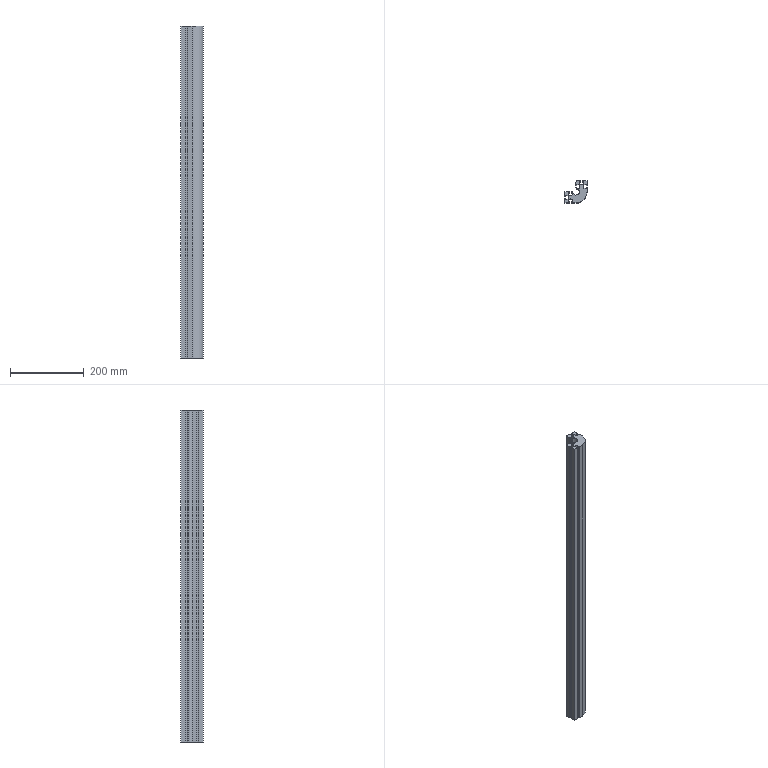Part | SolidWorks | features Extrusion 1 | 1 solid | 59 faces | box 60 x 60 x 900 mm | volume 1580758 mm3 | plane 50 | cylinder 9 | commonest cylinder face diameters 15.006 x7 18 x1 60 x1